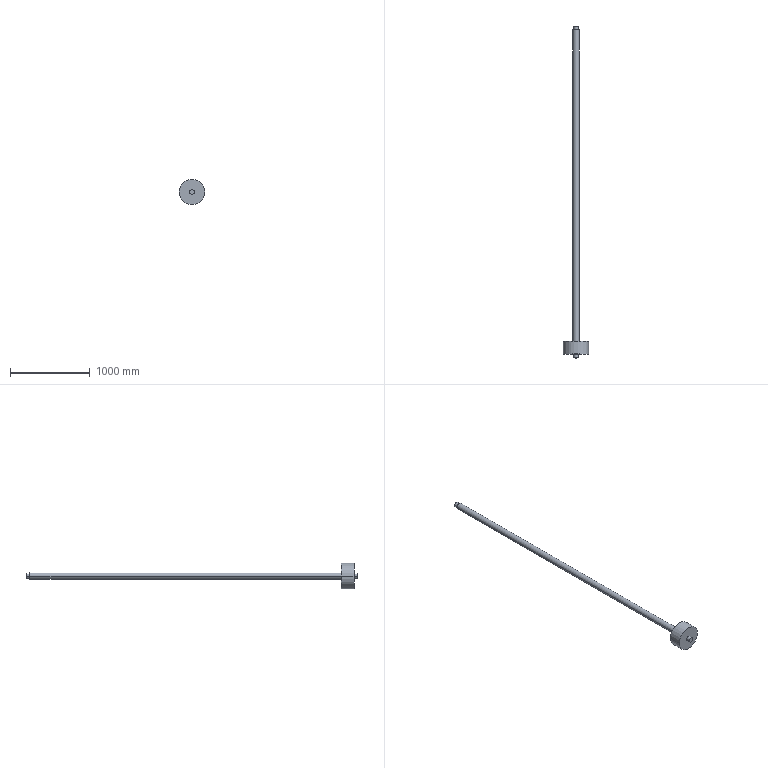Part | SolidWorks | features Revolution 1 | 1 solid | 13 faces | box 320 x 4176 x 320 mm | volume 32834670 mm3 | cylinder 8 | plane 5 | commonest cylinder face diameters 60 x4 80 x2 320 x2
STEP:
#1=CARTESIAN_POINT('',(-30.,4126.,0.));
#2=VERTEX_POINT('',#1);
#3=CARTESIAN_POINT('',(30.,4126.,0.));
#4=VERTEX_POINT('',#3);
#5=CARTESIAN_POINT('',(0.,4126.,0.));
#6=DIRECTION('',(0.,1.,0.));
#7=DIRECTION('',(-1.,0.,0.));
#8=AXIS2_PLACEMENT_3D('',#5,#6,#7);
#9=CIRCLE('',#8,30.);
#10=EDGE_CURVE('',#2,#4,#9,.T.);
#11=ORIENTED_EDGE('',*,*,#10,.T.);
#12=CARTESIAN_POINT('',(30.,4176.,0.));
#13=VERTEX_POINT('',#12);
#14=CARTESIAN_POINT('',(30.,4176.,0.));
#15=DIRECTION('',(0.,1.,0.));
#16=VECTOR('',#15,1000.);
#17=LINE('',#14,#16);
#18=EDGE_CURVE('',#4,#13,#17,.T.);
#19=ORIENTED_EDGE('',*,*,#18,.T.);
#20=CARTESIAN_POINT('',(-30.,4176.,0.));
#21=VERTEX_POINT('',#20);
#22=CARTESIAN_POINT('',(0.,4176.,0.));
#23=DIRECTION('',(0.,1.,0.));
#24=DIRECTION('',(-1.,0.,0.));
#25=AXIS2_PLACEMENT_3D('',#22,#23,#24);
#26=CIRCLE('',#25,30.);
#27=EDGE_CURVE('',#21,#13,#26,.T.);
#28=ORIENTED_EDGE('',*,*,#27,.F.);
#29=CARTESIAN_POINT('',(-30.,4176.,0.));
#30=DIRECTION('',(0.,1.,0.));
#31=VECTOR('',#30,1000.);
#32=LINE('',#29,#31);
#33=EDGE_CURVE('',#2,#21,#32,.T.);
#34=ORIENTED_EDGE('',*,*,#33,.F.);
#35=EDGE_LOOP('',(#11,#19,#28,#34));
#36=FACE_OUTER_BOUND('',#35,.T.);
#37=CARTESIAN_POINT('',(0.,4176.,0.));
#38=DIRECTION('',(0.,1.,0.));
#39=DIRECTION('',(-1.,0.,0.));
#40=AXIS2_PLACEMENT_3D('',#37,#38,#39);
#41=CYLINDRICAL_SURFACE('',#40,30.);
#42=ADVANCED_FACE('',(#36),#41,.T.);
#43=CARTESIAN_POINT('',(-40.,210.,0.));
#44=VERTEX_POINT('',#43);
#45=CARTESIAN_POINT('',(40.,210.,0.));
#46=VERTEX_POINT('',#45);
#47=CARTESIAN_POINT('',(0.,210.,0.));
#48=DIRECTION('',(0.,1.,0.));
#49=DIRECTION('',(-1.,0.,0.));
#50=AXIS2_PLACEMENT_3D('',#47,#48,#49);
#51=CIRCLE('',#50,40.);
#52=EDGE_CURVE('',#44,#46,#51,.T.);
#53=ORIENTED_EDGE('',*,*,#52,.T.);
#54=CARTESIAN_POINT('',(40.,4126.,0.));
#55=VERTEX_POINT('',#54);
#56=CARTESIAN_POINT('',(40.,4176.,0.));
#57=DIRECTION('',(0.,1.,0.));
#58=VECTOR('',#57,1000.);
#59=LINE('',#56,#58);
#60=EDGE_CURVE('',#46,#55,#59,.T.);
#61=ORIENTED_EDGE('',*,*,#60,.T.);
#62=CARTESIAN_POINT('',(-40.,4126.,0.));
#63=VERTEX_POINT('',#62);
#64=CARTESIAN_POINT('',(0.,4126.,0.));
#65=DIRECTION('',(0.,1.,0.));
#66=DIRECTION('',(-1.,0.,0.));
#67=AXIS2_PLACEMENT_3D('',#64,#65,#66);
#68=CIRCLE('',#67,40.);
#69=EDGE_CURVE('',#63,#55,#68,.T.);
#70=ORIENTED_EDGE('',*,*,#69,.F.);
#71=CARTESIAN_POINT('',(-40.,4176.,0.));
#72=DIRECTION('',(0.,1.,0.));
#73=VECTOR('',#72,1000.);
#74=LINE('',#71,#73);
#75=EDGE_CURVE('',#44,#63,#74,.T.);
#76=ORIENTED_EDGE('',*,*,#75,.F.);
#77=EDGE_LOOP('',(#53,#61,#70,#76));
#78=FACE_OUTER_BOUND('',#77,.T.);
#79=CARTESIAN_POINT('',(0.,4176.,0.));
#80=DIRECTION('',(0.,1.,0.));
#81=DIRECTION('',(-1.,0.,0.));
#82=AXIS2_PLACEMENT_3D('',#79,#80,#81);
#83=CYLINDRICAL_SURFACE('',#82,40.);
#84=ADVANCED_FACE('',(#78),#83,.T.);
#85=CARTESIAN_POINT('',(-160.,50.,0.));
#86=VERTEX_POINT('',#85);
#87=CARTESIAN_POINT('',(160.,50.,0.));
#88=VERTEX_POINT('',#87);
#89=CARTESIAN_POINT('',(0.,50.,0.));
#90=DIRECTION('',(0.,1.,0.));
#91=DIRECTION('',(-1.,0.,0.));
#92=AXIS2_PLACEMENT_3D('',#89,#90,#91);
#93=CIRCLE('',#92,160.);
#94=EDGE_CURVE('',#86,#88,#93,.T.);
#95=ORIENTED_EDGE('',*,*,#94,.T.);
#96=CARTESIAN_POINT('',(160.,210.,0.));
#97=VERTEX_POINT('',#96);
#98=CARTESIAN_POINT('',(160.,4176.,0.));
#99=DIRECTION('',(0.,1.,0.));
#100=VECTOR('',#99,1000.);
#101=LINE('',#98,#100);
#102=EDGE_CURVE('',#88,#97,#101,.T.);
#103=ORIENTED_EDGE('',*,*,#102,.T.);
#104=CARTESIAN_POINT('',(-160.,210.,0.));
#105=VERTEX_POINT('',#104);
#106=CARTESIAN_POINT('',(0.,210.,0.));
#107=DIRECTION('',(0.,1.,0.));
#108=DIRECTION('',(-1.,0.,0.));
#109=AXIS2_PLACEMENT_3D('',#106,#107,#108);
#110=CIRCLE('',#109,160.);
#111=EDGE_CURVE('',#105,#97,#110,.T.);
#112=ORIENTED_EDGE('',*,*,#111,.F.);
#113=CARTESIAN_POINT('',(-160.,4176.,0.));
#114=DIRECTION('',(0.,1.,0.));
#115=VECTOR('',#114,1000.);
#116=LINE('',#113,#115);
#117=EDGE_CURVE('',#86,#105,#116,.T.);
#118=ORIENTED_EDGE('',*,*,#117,.F.);
#119=EDGE_LOOP('',(#95,#103,#112,#118));
#120=FACE_OUTER_BOUND('',#119,.T.);
#121=CARTESIAN_POINT('',(0.,4176.,0.));
#122=DIRECTION('',(0.,1.,0.));
#123=DIRECTION('',(-1.,0.,0.));
#124=AXIS2_PLACEMENT_3D('',#121,#122,#123);
#125=CYLINDRICAL_SURFACE('',#124,160.);
#126=ADVANCED_FACE('',(#120),#125,.T.);
#127=CARTESIAN_POINT('',(-30.,0.,0.));
#128=VERTEX_POINT('',#127);
#129=CARTESIAN_POINT('',(30.,0.,0.));
#130=VERTEX_POINT('',#129);
#131=CARTESIAN_POINT('',(0.,0.,0.));
#132=DIRECTION('',(0.,1.,0.));
#133=DIRECTION('',(-1.,0.,0.));
#134=AXIS2_PLACEMENT_3D('',#131,#132,#133);
#135=CIRCLE('',#134,30.);
#136=EDGE_CURVE('',#128,#130,#135,.T.);
#137=ORIENTED_EDGE('',*,*,#136,.T.);
#138=CARTESIAN_POINT('',(30.,50.,0.));
#139=VERTEX_POINT('',#138);
#140=CARTESIAN_POINT('',(30.,4176.,0.));
#141=DIRECTION('',(0.,1.,0.));
#142=VECTOR('',#141,1000.);
#143=LINE('',#140,#142);
#144=EDGE_CURVE('',#130,#139,#143,.T.);
#145=ORIENTED_EDGE('',*,*,#144,.T.);
#146=CARTESIAN_POINT('',(-30.,50.,0.));
#147=VERTEX_POINT('',#146);
#148=CARTESIAN_POINT('',(0.,50.,0.));
#149=DIRECTION('',(0.,1.,0.));
#150=DIRECTION('',(-1.,0.,0.));
#151=AXIS2_PLACEMENT_3D('',#148,#149,#150);
#152=CIRCLE('',#151,30.);
#153=EDGE_CURVE('',#147,#139,#152,.T.);
#154=ORIENTED_EDGE('',*,*,#153,.F.);
#155=CARTESIAN_POINT('',(-30.,4176.,0.));
#156=DIRECTION('',(0.,1.,0.));
#157=VECTOR('',#156,1000.);
#158=LINE('',#155,#157);
#159=EDGE_CURVE('',#128,#147,#158,.T.);
#160=ORIENTED_EDGE('',*,*,#159,.F.);
#161=EDGE_LOOP('',(#137,#145,#154,#160));
#162=FACE_OUTER_BOUND('',#161,.T.);
#163=CARTESIAN_POINT('',(0.,4176.,0.));
#164=DIRECTION('',(0.,1.,0.));
#165=DIRECTION('',(-1.,0.,0.));
#166=AXIS2_PLACEMENT_3D('',#163,#164,#165);
#167=CYLINDRICAL_SURFACE('',#166,30.);
#168=ADVANCED_FACE('',(#162),#167,.T.);
#169=ORIENTED_EDGE('',*,*,#136,.F.);
#170=CARTESIAN_POINT('',(0.,0.,0.));
#171=DIRECTION('',(0.,1.,0.));
#172=DIRECTION('',(-1.,0.,0.));
#173=AXIS2_PLACEMENT_3D('',#170,#171,#172);
#174=CIRCLE('',#173,30.);
#175=EDGE_CURVE('',#130,#128,#174,.T.);
#176=ORIENTED_EDGE('',*,*,#175,.F.);
#177=EDGE_LOOP('',(#169,#176));
#178=FACE_OUTER_BOUND('',#177,.T.);
#179=CARTESIAN_POINT('',(0.,0.,0.));
#180=DIRECTION('',(0.,1.,0.));
#181=DIRECTION('',(-1.,0.,0.));
#182=AXIS2_PLACEMENT_3D('',#179,#180,#181);
#183=PLANE('',#182);
#184=ADVANCED_FACE('',(#178),#183,.F.);
#185=ORIENTED_EDGE('',*,*,#144,.F.);
#186=ORIENTED_EDGE('',*,*,#175,.T.);
#187=ORIENTED_EDGE('',*,*,#159,.T.);
#188=CARTESIAN_POINT('',(0.,50.,0.));
#189=DIRECTION('',(0.,1.,0.));
#190=DIRECTION('',(-1.,0.,0.));
#191=AXIS2_PLACEMENT_3D('',#188,#189,#190);
#192=CIRCLE('',#191,30.);
#193=EDGE_CURVE('',#139,#147,#192,.T.);
#194=ORIENTED_EDGE('',*,*,#193,.F.);
#195=EDGE_LOOP('',(#185,#186,#187,#194));
#196=FACE_OUTER_BOUND('',#195,.T.);
#197=CARTESIAN_POINT('',(0.,4176.,0.));
#198=DIRECTION('',(0.,1.,0.));
#199=DIRECTION('',(-1.,0.,0.));
#200=AXIS2_PLACEMENT_3D('',#197,#198,#199);
#201=CYLINDRICAL_SURFACE('',#200,30.);
#202=ADVANCED_FACE('',(#196),#201,.T.);
#203=ORIENTED_EDGE('',*,*,#94,.F.);
#204=CARTESIAN_POINT('',(0.,50.,0.));
#205=DIRECTION('',(0.,1.,0.));
#206=DIRECTION('',(-1.,0.,0.));
#207=AXIS2_PLACEMENT_3D('',#204,#205,#206);
#208=CIRCLE('',#207,160.);
#209=EDGE_CURVE('',#88,#86,#208,.T.);
#210=ORIENTED_EDGE('',*,*,#209,.F.);
#211=EDGE_LOOP('',(#203,#210));
#212=FACE_OUTER_BOUND('',#211,.T.);
#213=ORIENTED_EDGE('',*,*,#153,.T.);
#214=ORIENTED_EDGE('',*,*,#193,.T.);
#215=EDGE_LOOP('',(#213,#214));
#216=FACE_BOUND('',#215,.T.);
#217=CARTESIAN_POINT('',(30.,50.,0.));
#218=DIRECTION('',(0.,1.,0.));
#219=DIRECTION('',(-1.,0.,0.));
#220=AXIS2_PLACEMENT_3D('',#217,#218,#219);
#221=PLANE('',#220);
#222=ADVANCED_FACE('',(#212,#216),#221,.F.);
#223=ORIENTED_EDGE('',*,*,#102,.F.);
#224=ORIENTED_EDGE('',*,*,#209,.T.);
#225=ORIENTED_EDGE('',*,*,#117,.T.);
#226=CARTESIAN_POINT('',(0.,210.,0.));
#227=DIRECTION('',(0.,1.,0.));
#228=DIRECTION('',(-1.,0.,0.));
#229=AXIS2_PLACEMENT_3D('',#226,#227,#228);
#230=CIRCLE('',#229,160.);
#231=EDGE_CURVE('',#97,#105,#230,.T.);
#232=ORIENTED_EDGE('',*,*,#231,.F.);
#233=EDGE_LOOP('',(#223,#224,#225,#232));
#234=FACE_OUTER_BOUND('',#233,.T.);
#235=CARTESIAN_POINT('',(0.,4176.,0.));
#236=DIRECTION('',(0.,1.,0.));
#237=DIRECTION('',(-1.,0.,0.));
#238=AXIS2_PLACEMENT_3D('',#235,#236,#237);
#239=CYLINDRICAL_SURFACE('',#238,160.);
#240=ADVANCED_FACE('',(#234),#239,.T.);
#241=ORIENTED_EDGE('',*,*,#52,.F.);
#242=CARTESIAN_POINT('',(0.,210.,0.));
#243=DIRECTION('',(0.,1.,0.));
#244=DIRECTION('',(-1.,0.,0.));
#245=AXIS2_PLACEMENT_3D('',#242,#243,#244);
#246=CIRCLE('',#245,40.);
#247=EDGE_CURVE('',#46,#44,#246,.T.);
#248=ORIENTED_EDGE('',*,*,#247,.F.);
#249=EDGE_LOOP('',(#241,#248));
#250=FACE_BOUND('',#249,.T.);
#251=ORIENTED_EDGE('',*,*,#111,.T.);
#252=ORIENTED_EDGE('',*,*,#231,.T.);
#253=EDGE_LOOP('',(#251,#252));
#254=FACE_OUTER_BOUND('',#253,.T.);
#255=CARTESIAN_POINT('',(160.,210.,0.));
#256=DIRECTION('',(0.,-1.,0.));
#257=DIRECTION('',(1.,0.,0.));
#258=AXIS2_PLACEMENT_3D('',#255,#256,#257);
#259=PLANE('',#258);
#260=ADVANCED_FACE('',(#250,#254),#259,.F.);
#261=ORIENTED_EDGE('',*,*,#60,.F.);
#262=ORIENTED_EDGE('',*,*,#247,.T.);
#263=ORIENTED_EDGE('',*,*,#75,.T.);
#264=CARTESIAN_POINT('',(0.,4126.,0.));
#265=DIRECTION('',(0.,1.,0.));
#266=DIRECTION('',(-1.,0.,0.));
#267=AXIS2_PLACEMENT_3D('',#264,#265,#266);
#268=CIRCLE('',#267,40.);
#269=EDGE_CURVE('',#55,#63,#268,.T.);
#270=ORIENTED_EDGE('',*,*,#269,.F.);
#271=EDGE_LOOP('',(#261,#262,#263,#270));
#272=FACE_OUTER_BOUND('',#271,.T.);
#273=CARTESIAN_POINT('',(0.,4176.,0.));
#274=DIRECTION('',(0.,1.,0.));
#275=DIRECTION('',(-1.,0.,0.));
#276=AXIS2_PLACEMENT_3D('',#273,#274,#275);
#277=CYLINDRICAL_SURFACE('',#276,40.);
#278=ADVANCED_FACE('',(#272),#277,.T.);
#279=ORIENTED_EDGE('',*,*,#10,.F.);
#280=CARTESIAN_POINT('',(0.,4126.,0.));
#281=DIRECTION('',(0.,1.,0.));
#282=DIRECTION('',(-1.,0.,0.));
#283=AXIS2_PLACEMENT_3D('',#280,#281,#282);
#284=CIRCLE('',#283,30.);
#285=EDGE_CURVE('',#4,#2,#284,.T.);
#286=ORIENTED_EDGE('',*,*,#285,.F.);
#287=EDGE_LOOP('',(#279,#286));
#288=FACE_BOUND('',#287,.T.);
#289=ORIENTED_EDGE('',*,*,#69,.T.);
#290=ORIENTED_EDGE('',*,*,#269,.T.);
#291=EDGE_LOOP('',(#289,#290));
#292=FACE_OUTER_BOUND('',#291,.T.);
#293=CARTESIAN_POINT('',(40.,4126.,0.));
#294=DIRECTION('',(0.,-1.,0.));
#295=DIRECTION('',(1.,0.,0.));
#296=AXIS2_PLACEMENT_3D('',#293,#294,#295);
#297=PLANE('',#296);
#298=ADVANCED_FACE('',(#288,#292),#297,.F.);
#299=ORIENTED_EDGE('',*,*,#18,.F.);
#300=ORIENTED_EDGE('',*,*,#285,.T.);
#301=ORIENTED_EDGE('',*,*,#33,.T.);
#302=CARTESIAN_POINT('',(0.,4176.,0.));
#303=DIRECTION('',(0.,1.,0.));
#304=DIRECTION('',(-1.,0.,0.));
#305=AXIS2_PLACEMENT_3D('',#302,#303,#304);
#306=CIRCLE('',#305,30.);
#307=EDGE_CURVE('',#13,#21,#306,.T.);
#308=ORIENTED_EDGE('',*,*,#307,.F.);
#309=EDGE_LOOP('',(#299,#300,#301,#308));
#310=FACE_OUTER_BOUND('',#309,.T.);
#311=CARTESIAN_POINT('',(0.,4176.,0.));
#312=DIRECTION('',(0.,1.,0.));
#313=DIRECTION('',(-1.,0.,0.));
#314=AXIS2_PLACEMENT_3D('',#311,#312,#313);
#315=CYLINDRICAL_SURFACE('',#314,30.);
#316=ADVANCED_FACE('',(#310),#315,.T.);
#317=ORIENTED_EDGE('',*,*,#27,.T.);
#318=ORIENTED_EDGE('',*,*,#307,.T.);
#319=EDGE_LOOP('',(#317,#318));
#320=FACE_OUTER_BOUND('',#319,.T.);
#321=CARTESIAN_POINT('',(30.,4176.,0.));
#322=DIRECTION('',(0.,-1.,0.));
#323=DIRECTION('',(1.,0.,0.));
#324=AXIS2_PLACEMENT_3D('',#321,#322,#323);
#325=PLANE('',#324);
#326=ADVANCED_FACE('',(#320),#325,.F.);
#327=CLOSED_SHELL('',(#42,#84,#126,#168,#184,#202,#222,#240,#260,#278,#298,#316,#326));
#328=MANIFOLD_SOLID_BREP('',#327);
#329=CARTESIAN_POINT('',(0.,0.,0.));
#330=DIRECTION('',(0.,0.,1.));
#331=DIRECTION('',(1.,0.,0.));
#332=AXIS2_PLACEMENT_3D('',#329,#330,#331);
#333=(LENGTH_UNIT()NAMED_UNIT(*)SI_UNIT(.MILLI.,.METRE.));
#334=UNCERTAINTY_MEASURE_WITH_UNIT(LENGTH_MEASURE(0.00001),#333,'','');
#335=(NAMED_UNIT(*)PLANE_ANGLE_UNIT()SI_UNIT($,.RADIAN.));
#336=(NAMED_UNIT(*)SI_UNIT($,.STERADIAN.)SOLID_ANGLE_UNIT());
#337=(GEOMETRIC_REPRESENTATION_CONTEXT(3)GLOBAL_UNCERTAINTY_ASSIGNED_CONTEXT((#334))GLOBAL_UNIT_ASSIGNED_CONTEXT((#333,#335,#336))REPRESENTATION_CONTEXT('',''));
#338=ADVANCED_BREP_SHAPE_REPRESENTATION('',(#328,#332),#337);